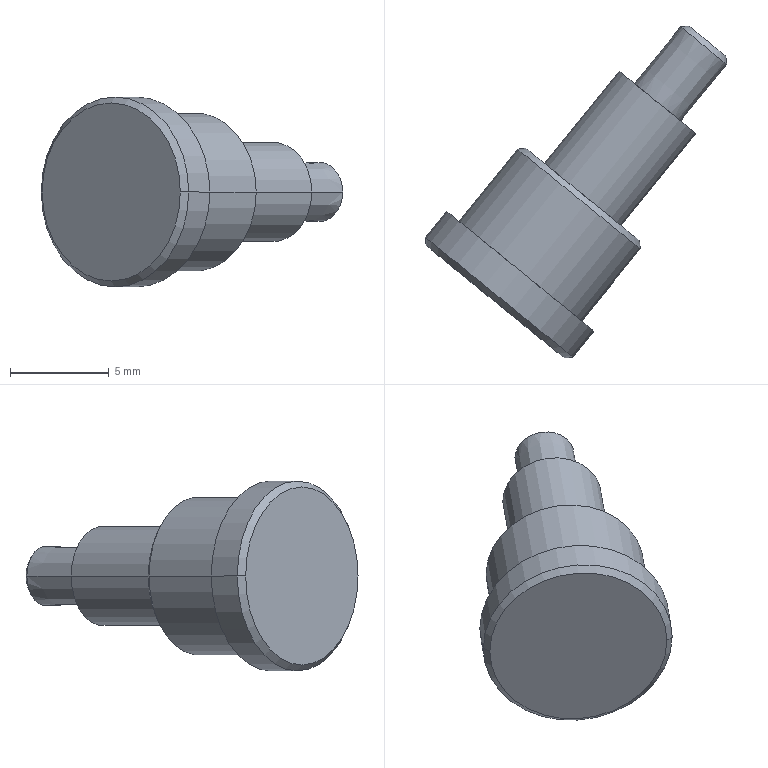Part | SolidWorks | features BaseBody 1 | 1 solid | 19 faces | box 15.235 x 16.785 x 9.6 mm | volume 539.336 mm3 | cone 8 | cylinder 6 | plane 5 | commonest cylinder face diameters 5 x2 8 x2 9.6 x2
STEP:
#1=CARTESIAN_POINT('',(528.138,-164.807,289.195));
#2=VERTEX_POINT('',#1);
#3=CARTESIAN_POINT('',(521.155,-159.129,289.195));
#4=VERTEX_POINT('',#3);
#5=CARTESIAN_POINT('',(524.647,-161.968,289.195));
#6=DIRECTION('',(-0.6309,-0.7758,0.000000012));
#7=DIRECTION('',(-0.7758,0.6309,0.));
#8=AXIS2_PLACEMENT_3D('',#5,#6,#7);
#9=CIRCLE('',#8,4.5);
#10=EDGE_CURVE('',#2,#4,#9,.T.);
#11=ORIENTED_EDGE('',*,*,#10,.F.);
#12=CARTESIAN_POINT('',(528.56,-164.764,289.195));
#13=VERTEX_POINT('',#12);
#14=CARTESIAN_POINT('',(528.56,-164.764,289.195));
#15=DIRECTION('',(0.9947,0.1025,-0.000000009));
#16=VECTOR('',#15,1000.);
#17=LINE('',#14,#16);
#18=EDGE_CURVE('',#2,#13,#17,.T.);
#19=ORIENTED_EDGE('',*,*,#18,.T.);
#20=CARTESIAN_POINT('',(521.112,-158.707,289.195));
#21=VERTEX_POINT('',#20);
#22=CARTESIAN_POINT('',(524.836,-161.736,289.195));
#23=DIRECTION('',(-0.6309,-0.7758,0.000000012));
#24=DIRECTION('',(0.7758,-0.6309,-0.000000021));
#25=AXIS2_PLACEMENT_3D('',#22,#23,#24);
#26=CIRCLE('',#25,4.8);
#27=EDGE_CURVE('',#13,#21,#26,.T.);
#28=ORIENTED_EDGE('',*,*,#27,.T.);
#29=CARTESIAN_POINT('',(521.112,-158.707,289.195));
#30=DIRECTION('',(-0.1025,0.9947,-0.000000009));
#31=VECTOR('',#30,1000.);
#32=LINE('',#29,#31);
#33=EDGE_CURVE('',#4,#21,#32,.T.);
#34=ORIENTED_EDGE('',*,*,#33,.F.);
#35=EDGE_LOOP('',(#11,#19,#28,#34));
#36=FACE_OUTER_BOUND('',#35,.T.);
#37=CARTESIAN_POINT('',(524.836,-161.736,289.195));
#38=DIRECTION('',(0.6309,0.7758,-0.000000012));
#39=DIRECTION('',(-0.7758,0.6309,0.));
#40=AXIS2_PLACEMENT_3D('',#37,#38,#39);
#41=CONICAL_SURFACE('',#40,4.8,0.7854);
#42=ADVANCED_FACE('',(#36),#41,.T.);
#43=ORIENTED_EDGE('',*,*,#27,.F.);
#44=CARTESIAN_POINT('',(529.633,-163.445,289.195));
#45=VERTEX_POINT('',#44);
#46=CARTESIAN_POINT('',(529.002,-164.221,289.195));
#47=DIRECTION('',(0.6309,0.7758,-0.000000012));
#48=VECTOR('',#47,1000.);
#49=LINE('',#46,#48);
#50=EDGE_CURVE('',#13,#45,#49,.T.);
#51=ORIENTED_EDGE('',*,*,#50,.T.);
#52=CARTESIAN_POINT('',(522.184,-157.388,289.195));
#53=VERTEX_POINT('',#52);
#54=CARTESIAN_POINT('',(525.908,-160.417,289.195));
#55=DIRECTION('',(-0.6309,-0.7758,0.000000012));
#56=DIRECTION('',(-0.7758,0.6309,0.));
#57=AXIS2_PLACEMENT_3D('',#54,#55,#56);
#58=CIRCLE('',#57,4.8);
#59=EDGE_CURVE('',#45,#53,#58,.T.);
#60=ORIENTED_EDGE('',*,*,#59,.T.);
#61=CARTESIAN_POINT('',(521.554,-158.164,289.195));
#62=DIRECTION('',(0.6309,0.7758,-0.000000012));
#63=VECTOR('',#62,1000.);
#64=LINE('',#61,#63);
#65=EDGE_CURVE('',#21,#53,#64,.T.);
#66=ORIENTED_EDGE('',*,*,#65,.F.);
#67=EDGE_LOOP('',(#43,#51,#60,#66));
#68=FACE_OUTER_BOUND('',#67,.T.);
#69=CARTESIAN_POINT('',(525.278,-161.192,289.195));
#70=DIRECTION('',(0.6309,0.7758,-0.000000012));
#71=DIRECTION('',(-0.7758,0.6309,0.));
#72=AXIS2_PLACEMENT_3D('',#69,#70,#71);
#73=CYLINDRICAL_SURFACE('',#72,4.8);
#74=ADVANCED_FACE('',(#68),#73,.T.);
#75=CARTESIAN_POINT('',(529.012,-162.94,289.195));
#76=VERTEX_POINT('',#75);
#77=CARTESIAN_POINT('',(522.805,-157.893,289.195));
#78=VERTEX_POINT('',#77);
#79=CARTESIAN_POINT('',(525.908,-160.417,289.195));
#80=DIRECTION('',(-0.6309,-0.7758,0.000000012));
#81=DIRECTION('',(-0.7758,0.6309,0.));
#82=AXIS2_PLACEMENT_3D('',#79,#80,#81);
#83=CIRCLE('',#82,4.);
#84=EDGE_CURVE('',#76,#78,#83,.T.);
#85=ORIENTED_EDGE('',*,*,#84,.F.);
#86=CARTESIAN_POINT('',(531.977,-159.294,289.195));
#87=VERTEX_POINT('',#86);
#88=CARTESIAN_POINT('',(530.589,-161.001,289.195));
#89=DIRECTION('',(0.6309,0.7758,-0.000000012));
#90=VECTOR('',#89,1000.);
#91=LINE('',#88,#90);
#92=EDGE_CURVE('',#76,#87,#91,.T.);
#93=ORIENTED_EDGE('',*,*,#92,.T.);
#94=CARTESIAN_POINT('',(525.77,-154.246,289.195));
#95=VERTEX_POINT('',#94);
#96=CARTESIAN_POINT('',(528.874,-156.77,289.195));
#97=DIRECTION('',(-0.6309,-0.7758,0.000000012));
#98=DIRECTION('',(-0.7758,0.6309,0.));
#99=AXIS2_PLACEMENT_3D('',#96,#97,#98);
#100=CIRCLE('',#99,4.);
#101=EDGE_CURVE('',#87,#95,#100,.T.);
#102=ORIENTED_EDGE('',*,*,#101,.T.);
#103=CARTESIAN_POINT('',(524.382,-155.953,289.195));
#104=DIRECTION('',(0.6309,0.7758,-0.000000012));
#105=VECTOR('',#104,1000.);
#106=LINE('',#103,#105);
#107=EDGE_CURVE('',#78,#95,#106,.T.);
#108=ORIENTED_EDGE('',*,*,#107,.F.);
#109=EDGE_LOOP('',(#85,#93,#102,#108));
#110=FACE_OUTER_BOUND('',#109,.T.);
#111=CARTESIAN_POINT('',(527.486,-158.477,289.195));
#112=DIRECTION('',(0.6309,0.7758,-0.000000012));
#113=DIRECTION('',(-0.7758,0.6309,0.));
#114=AXIS2_PLACEMENT_3D('',#111,#112,#113);
#115=CYLINDRICAL_SURFACE('',#114,4.);
#116=ADVANCED_FACE('',(#110),#115,.T.);
#117=CARTESIAN_POINT('',(531.934,-158.872,289.195));
#118=VERTEX_POINT('',#117);
#119=CARTESIAN_POINT('',(526.193,-154.203,289.195));
#120=VERTEX_POINT('',#119);
#121=CARTESIAN_POINT('',(529.063,-156.537,289.195));
#122=DIRECTION('',(-0.6309,-0.7758,0.000000012));
#123=DIRECTION('',(0.7758,-0.6309,0.));
#124=AXIS2_PLACEMENT_3D('',#121,#122,#123);
#125=CIRCLE('',#124,3.7);
#126=EDGE_CURVE('',#118,#120,#125,.T.);
#127=ORIENTED_EDGE('',*,*,#126,.T.);
#128=CARTESIAN_POINT('',(525.77,-154.246,289.195));
#129=DIRECTION('',(-0.9947,-0.1025,0.000000009));
#130=VECTOR('',#129,1000.);
#131=LINE('',#128,#130);
#132=EDGE_CURVE('',#120,#95,#131,.T.);
#133=ORIENTED_EDGE('',*,*,#132,.T.);
#134=ORIENTED_EDGE('',*,*,#101,.F.);
#135=CARTESIAN_POINT('',(531.977,-159.294,289.195));
#136=DIRECTION('',(0.1025,-0.9947,0.000000009));
#137=VECTOR('',#136,1000.);
#138=LINE('',#135,#137);
#139=EDGE_CURVE('',#118,#87,#138,.T.);
#140=ORIENTED_EDGE('',*,*,#139,.F.);
#141=EDGE_LOOP('',(#127,#133,#134,#140));
#142=FACE_OUTER_BOUND('',#141,.T.);
#143=CARTESIAN_POINT('',(528.874,-156.77,289.195));
#144=DIRECTION('',(-0.6309,-0.7758,0.000000012));
#145=DIRECTION('',(0.7758,-0.6309,0.));
#146=AXIS2_PLACEMENT_3D('',#143,#144,#145);
#147=CONICAL_SURFACE('',#146,4.,0.7854);
#148=ADVANCED_FACE('',(#142),#147,.T.);
#149=CARTESIAN_POINT('',(531.003,-158.115,289.195));
#150=VERTEX_POINT('',#149);
#151=CARTESIAN_POINT('',(527.124,-154.96,289.195));
#152=VERTEX_POINT('',#151);
#153=CARTESIAN_POINT('',(529.063,-156.537,289.195));
#154=DIRECTION('',(-0.6309,-0.7758,0.000000012));
#155=DIRECTION('',(-0.7758,0.6309,0.));
#156=AXIS2_PLACEMENT_3D('',#153,#154,#155);
#157=CIRCLE('',#156,2.5);
#158=EDGE_CURVE('',#150,#152,#157,.T.);
#159=ORIENTED_EDGE('',*,*,#158,.F.);
#160=CARTESIAN_POINT('',(534.788,-153.46,289.195));
#161=VERTEX_POINT('',#160);
#162=CARTESIAN_POINT('',(532.896,-155.787,289.195));
#163=DIRECTION('',(0.6309,0.7758,-0.000000012));
#164=VECTOR('',#163,1000.);
#165=LINE('',#162,#164);
#166=EDGE_CURVE('',#150,#161,#165,.T.);
#167=ORIENTED_EDGE('',*,*,#166,.T.);
#168=CARTESIAN_POINT('',(530.909,-150.305,289.195));
#169=VERTEX_POINT('',#168);
#170=CARTESIAN_POINT('',(532.849,-151.882,289.195));
#171=DIRECTION('',(-0.6309,-0.7758,0.000000012));
#172=DIRECTION('',(-0.7758,0.6309,0.));
#173=AXIS2_PLACEMENT_3D('',#170,#171,#172);
#174=CIRCLE('',#173,2.5);
#175=EDGE_CURVE('',#161,#169,#174,.T.);
#176=ORIENTED_EDGE('',*,*,#175,.T.);
#177=CARTESIAN_POINT('',(529.016,-152.633,289.195));
#178=DIRECTION('',(0.6309,0.7758,-0.000000012));
#179=VECTOR('',#178,1000.);
#180=LINE('',#177,#179);
#181=EDGE_CURVE('',#152,#169,#180,.T.);
#182=ORIENTED_EDGE('',*,*,#181,.F.);
#183=EDGE_LOOP('',(#159,#167,#176,#182));
#184=FACE_OUTER_BOUND('',#183,.T.);
#185=CARTESIAN_POINT('',(530.956,-154.21,289.195));
#186=DIRECTION('',(0.6309,0.7758,-0.000000012));
#187=DIRECTION('',(-0.7758,0.6309,0.));
#188=AXIS2_PLACEMENT_3D('',#185,#186,#187);
#189=CYLINDRICAL_SURFACE('',#188,2.5);
#190=ADVANCED_FACE('',(#184),#189,.T.);
#191=CARTESIAN_POINT('',(536.346,-149.958,289.195));
#192=VERTEX_POINT('',#191);
#193=CARTESIAN_POINT('',(534.02,-148.066,289.195));
#194=VERTEX_POINT('',#193);
#195=CARTESIAN_POINT('',(535.183,-149.012,289.195));
#196=DIRECTION('',(-0.6309,-0.7758,0.000000012));
#197=DIRECTION('',(0.7758,-0.6309,-0.000000021));
#198=AXIS2_PLACEMENT_3D('',#195,#196,#197);
#199=CIRCLE('',#198,1.499);
#200=EDGE_CURVE('',#192,#194,#199,.T.);
#201=ORIENTED_EDGE('',*,*,#200,.T.);
#202=CARTESIAN_POINT('',(531.685,-150.936,289.195));
#203=VERTEX_POINT('',#202);
#204=CARTESIAN_POINT('',(531.685,-150.936,289.195));
#205=DIRECTION('',(-0.6311,-0.7757,0.000000012));
#206=VECTOR('',#205,1000.);
#207=LINE('',#204,#206);
#208=EDGE_CURVE('',#194,#203,#207,.T.);
#209=ORIENTED_EDGE('',*,*,#208,.T.);
#210=CARTESIAN_POINT('',(534.012,-152.829,289.195));
#211=VERTEX_POINT('',#210);
#212=CARTESIAN_POINT('',(532.849,-151.882,289.195));
#213=DIRECTION('',(-0.6309,-0.7758,0.000000012));
#214=DIRECTION('',(0.7758,-0.6309,0.));
#215=AXIS2_PLACEMENT_3D('',#212,#213,#214);
#216=CIRCLE('',#215,1.5);
#217=EDGE_CURVE('',#211,#203,#216,.T.);
#218=ORIENTED_EDGE('',*,*,#217,.F.);
#219=CARTESIAN_POINT('',(534.012,-152.829,289.195));
#220=DIRECTION('',(-0.6308,-0.7759,0.000000012));
#221=VECTOR('',#220,1000.);
#222=LINE('',#219,#221);
#223=EDGE_CURVE('',#192,#211,#222,.T.);
#224=ORIENTED_EDGE('',*,*,#223,.F.);
#225=EDGE_LOOP('',(#201,#209,#218,#224));
#226=FACE_OUTER_BOUND('',#225,.T.);
#227=CARTESIAN_POINT('',(532.849,-151.882,289.195));
#228=DIRECTION('',(-0.6309,-0.7758,0.000000012));
#229=DIRECTION('',(0.7758,-0.6309,0.));
#230=AXIS2_PLACEMENT_3D('',#227,#228,#229);
#231=CONICAL_SURFACE('',#230,1.5,0.0001745);
#232=ADVANCED_FACE('',(#226),#231,.T.);
#233=CARTESIAN_POINT('',(536.303,-149.536,289.195));
#234=VERTEX_POINT('',#233);
#235=CARTESIAN_POINT('',(534.442,-148.022,289.195));
#236=VERTEX_POINT('',#235);
#237=CARTESIAN_POINT('',(535.372,-148.779,289.195));
#238=DIRECTION('',(-0.6309,-0.7758,0.000000012));
#239=DIRECTION('',(0.7758,-0.6309,0.));
#240=AXIS2_PLACEMENT_3D('',#237,#238,#239);
#241=CIRCLE('',#240,1.199);
#242=EDGE_CURVE('',#234,#236,#241,.T.);
#243=ORIENTED_EDGE('',*,*,#242,.T.);
#244=CARTESIAN_POINT('',(534.02,-148.066,289.195));
#245=DIRECTION('',(-0.9947,-0.1024,0.000000009));
#246=VECTOR('',#245,1000.);
#247=LINE('',#244,#246);
#248=EDGE_CURVE('',#236,#194,#247,.T.);
#249=ORIENTED_EDGE('',*,*,#248,.T.);
#250=ORIENTED_EDGE('',*,*,#200,.F.);
#251=CARTESIAN_POINT('',(536.346,-149.958,289.195));
#252=DIRECTION('',(0.1026,-0.9947,0.000000009));
#253=VECTOR('',#252,1000.);
#254=LINE('',#251,#253);
#255=EDGE_CURVE('',#234,#192,#254,.T.);
#256=ORIENTED_EDGE('',*,*,#255,.F.);
#257=EDGE_LOOP('',(#243,#249,#250,#256));
#258=FACE_OUTER_BOUND('',#257,.T.);
#259=CARTESIAN_POINT('',(535.183,-149.012,289.195));
#260=DIRECTION('',(-0.6309,-0.7758,0.000000012));
#261=DIRECTION('',(0.7758,-0.6309,0.));
#262=AXIS2_PLACEMENT_3D('',#259,#260,#261);
#263=CONICAL_SURFACE('',#262,1.499,0.7855);
#264=ADVANCED_FACE('',(#258),#263,.T.);
#265=CARTESIAN_POINT('',(524.647,-161.968,289.195));
#266=DIRECTION('',(-0.6309,-0.7758,0.000000012));
#267=DIRECTION('',(-0.7758,0.6309,0.));
#268=AXIS2_PLACEMENT_3D('',#265,#266,#267);
#269=CIRCLE('',#268,4.5);
#270=EDGE_CURVE('',#4,#2,#269,.T.);
#271=ORIENTED_EDGE('',*,*,#270,.T.);
#272=ORIENTED_EDGE('',*,*,#10,.T.);
#273=EDGE_LOOP('',(#271,#272));
#274=FACE_OUTER_BOUND('',#273,.T.);
#275=CARTESIAN_POINT('',(526.509,-163.482,289.195));
#276=DIRECTION('',(-0.6309,-0.7758,0.000000012));
#277=DIRECTION('',(0.7758,-0.6309,0.));
#278=AXIS2_PLACEMENT_3D('',#275,#276,#277);
#279=PLANE('',#278);
#280=ADVANCED_FACE('',(#274),#279,.T.);
#281=ORIENTED_EDGE('',*,*,#18,.F.);
#282=ORIENTED_EDGE('',*,*,#270,.F.);
#283=ORIENTED_EDGE('',*,*,#33,.T.);
#284=CARTESIAN_POINT('',(524.836,-161.736,289.195));
#285=DIRECTION('',(-0.6309,-0.7758,0.000000012));
#286=DIRECTION('',(0.7758,-0.6309,-0.000000021));
#287=AXIS2_PLACEMENT_3D('',#284,#285,#286);
#288=CIRCLE('',#287,4.8);
#289=EDGE_CURVE('',#21,#13,#288,.T.);
#290=ORIENTED_EDGE('',*,*,#289,.T.);
#291=EDGE_LOOP('',(#281,#282,#283,#290));
#292=FACE_OUTER_BOUND('',#291,.T.);
#293=CARTESIAN_POINT('',(524.836,-161.736,289.195));
#294=DIRECTION('',(0.6309,0.7758,-0.000000012));
#295=DIRECTION('',(-0.7758,0.6309,0.));
#296=AXIS2_PLACEMENT_3D('',#293,#294,#295);
#297=CONICAL_SURFACE('',#296,4.8,0.7854);
#298=ADVANCED_FACE('',(#292),#297,.T.);
#299=ORIENTED_EDGE('',*,*,#50,.F.);
#300=ORIENTED_EDGE('',*,*,#289,.F.);
#301=ORIENTED_EDGE('',*,*,#65,.T.);
#302=CARTESIAN_POINT('',(525.908,-160.417,289.195));
#303=DIRECTION('',(-0.6309,-0.7758,0.000000012));
#304=DIRECTION('',(-0.7758,0.6309,0.));
#305=AXIS2_PLACEMENT_3D('',#302,#303,#304);
#306=CIRCLE('',#305,4.8);
#307=EDGE_CURVE('',#53,#45,#306,.T.);
#308=ORIENTED_EDGE('',*,*,#307,.T.);
#309=EDGE_LOOP('',(#299,#300,#301,#308));
#310=FACE_OUTER_BOUND('',#309,.T.);
#311=CARTESIAN_POINT('',(525.278,-161.192,289.195));
#312=DIRECTION('',(0.6309,0.7758,-0.000000012));
#313=DIRECTION('',(-0.7758,0.6309,0.));
#314=AXIS2_PLACEMENT_3D('',#311,#312,#313);
#315=CYLINDRICAL_SURFACE('',#314,4.8);
#316=ADVANCED_FACE('',(#310),#315,.T.);
#317=CARTESIAN_POINT('',(525.908,-160.417,289.195));
#318=DIRECTION('',(-0.6309,-0.7758,0.000000012));
#319=DIRECTION('',(-0.7758,0.6309,0.));
#320=AXIS2_PLACEMENT_3D('',#317,#318,#319);
#321=CIRCLE('',#320,4.);
#322=EDGE_CURVE('',#78,#76,#321,.T.);
#323=ORIENTED_EDGE('',*,*,#322,.T.);
#324=ORIENTED_EDGE('',*,*,#84,.T.);
#325=EDGE_LOOP('',(#323,#324));
#326=FACE_BOUND('',#325,.T.);
#327=ORIENTED_EDGE('',*,*,#307,.F.);
#328=ORIENTED_EDGE('',*,*,#59,.F.);
#329=EDGE_LOOP('',(#327,#328));
#330=FACE_OUTER_BOUND('',#329,.T.);
#331=CARTESIAN_POINT('',(529.322,-163.193,289.195));
#332=DIRECTION('',(0.6309,0.7758,-0.000000012));
#333=DIRECTION('',(-0.7758,0.6309,0.));
#334=AXIS2_PLACEMENT_3D('',#331,#332,#333);
#335=PLANE('',#334);
#336=ADVANCED_FACE('',(#326,#330),#335,.T.);
#337=ORIENTED_EDGE('',*,*,#92,.F.);
#338=ORIENTED_EDGE('',*,*,#322,.F.);
#339=ORIENTED_EDGE('',*,*,#107,.T.);
#340=CARTESIAN_POINT('',(528.874,-156.77,289.195));
#341=DIRECTION('',(-0.6309,-0.7758,0.000000012));
#342=DIRECTION('',(-0.7758,0.6309,0.));
#343=AXIS2_PLACEMENT_3D('',#340,#341,#342);
#344=CIRCLE('',#343,4.);
#345=EDGE_CURVE('',#95,#87,#344,.T.);
#346=ORIENTED_EDGE('',*,*,#345,.T.);
#347=EDGE_LOOP('',(#337,#338,#339,#346));
#348=FACE_OUTER_BOUND('',#347,.T.);
#349=CARTESIAN_POINT('',(527.486,-158.477,289.195));
#350=DIRECTION('',(0.6309,0.7758,-0.000000012));
#351=DIRECTION('',(-0.7758,0.6309,0.));
#352=AXIS2_PLACEMENT_3D('',#349,#350,#351);
#353=CYLINDRICAL_SURFACE('',#352,4.);
#354=ADVANCED_FACE('',(#348),#353,.T.);
#355=ORIENTED_EDGE('',*,*,#132,.F.);
#356=CARTESIAN_POINT('',(529.063,-156.537,289.195));
#357=DIRECTION('',(-0.6309,-0.7758,0.000000012));
#358=DIRECTION('',(0.7758,-0.6309,0.));
#359=AXIS2_PLACEMENT_3D('',#356,#357,#358);
#360=CIRCLE('',#359,3.7);
#361=EDGE_CURVE('',#120,#118,#360,.T.);
#362=ORIENTED_EDGE('',*,*,#361,.T.);
#363=ORIENTED_EDGE('',*,*,#139,.T.);
#364=ORIENTED_EDGE('',*,*,#345,.F.);
#365=EDGE_LOOP('',(#355,#362,#363,#364));
#366=FACE_OUTER_BOUND('',#365,.T.);
#367=CARTESIAN_POINT('',(528.874,-156.77,289.195));
#368=DIRECTION('',(-0.6309,-0.7758,0.000000012));
#369=DIRECTION('',(0.7758,-0.6309,0.));
#370=AXIS2_PLACEMENT_3D('',#367,#368,#369);
#371=CONICAL_SURFACE('',#370,4.,0.7854);
#372=ADVANCED_FACE('',(#366),#371,.T.);
#373=ORIENTED_EDGE('',*,*,#126,.F.);
#374=ORIENTED_EDGE('',*,*,#361,.F.);
#375=EDGE_LOOP('',(#373,#374));
#376=FACE_OUTER_BOUND('',#375,.T.);
#377=CARTESIAN_POINT('',(529.063,-156.537,289.195));
#378=DIRECTION('',(-0.6309,-0.7758,0.000000012));
#379=DIRECTION('',(-0.7758,0.6309,0.));
#380=AXIS2_PLACEMENT_3D('',#377,#378,#379);
#381=CIRCLE('',#380,2.5);
#382=EDGE_CURVE('',#152,#150,#381,.T.);
#383=ORIENTED_EDGE('',*,*,#382,.T.);
#384=ORIENTED_EDGE('',*,*,#158,.T.);
#385=EDGE_LOOP('',(#383,#384));
#386=FACE_BOUND('',#385,.T.);
#387=CARTESIAN_POINT('',(531.585,-158.588,289.195));
#388=DIRECTION('',(0.6309,0.7758,-0.000000012));
#389=DIRECTION('',(-0.7758,0.6309,0.));
#390=AXIS2_PLACEMENT_3D('',#387,#388,#389);
#391=PLANE('',#390);
#392=ADVANCED_FACE('',(#376,#386),#391,.T.);
#393=ORIENTED_EDGE('',*,*,#166,.F.);
#394=ORIENTED_EDGE('',*,*,#382,.F.);
#395=ORIENTED_EDGE('',*,*,#181,.T.);
#396=CARTESIAN_POINT('',(532.849,-151.882,289.195));
#397=DIRECTION('',(-0.6309,-0.7758,0.000000012));
#398=DIRECTION('',(-0.7758,0.6309,0.));
#399=AXIS2_PLACEMENT_3D('',#396,#397,#398);
#400=CIRCLE('',#399,2.5);
#401=EDGE_CURVE('',#169,#161,#400,.T.);
#402=ORIENTED_EDGE('',*,*,#401,.T.);
#403=EDGE_LOOP('',(#393,#394,#395,#402));
#404=FACE_OUTER_BOUND('',#403,.T.);
#405=CARTESIAN_POINT('',(530.956,-154.21,289.195));
#406=DIRECTION('',(0.6309,0.7758,-0.000000012));
#407=DIRECTION('',(-0.7758,0.6309,0.));
#408=AXIS2_PLACEMENT_3D('',#405,#406,#407);
#409=CYLINDRICAL_SURFACE('',#408,2.5);
#410=ADVANCED_FACE('',(#404),#409,.T.);
#411=ORIENTED_EDGE('',*,*,#401,.F.);
#412=ORIENTED_EDGE('',*,*,#175,.F.);
#413=EDGE_LOOP('',(#411,#412));
#414=FACE_OUTER_BOUND('',#413,.T.);
#415=ORIENTED_EDGE('',*,*,#217,.T.);
#416=CARTESIAN_POINT('',(532.849,-151.882,289.195));
#417=DIRECTION('',(-0.6309,-0.7758,0.000000012));
#418=DIRECTION('',(0.7758,-0.6309,0.));
#419=AXIS2_PLACEMENT_3D('',#416,#417,#418);
#420=CIRCLE('',#419,1.5);
#421=EDGE_CURVE('',#203,#211,#420,.T.);
#422=ORIENTED_EDGE('',*,*,#421,.T.);
#423=EDGE_LOOP('',(#415,#422));
#424=FACE_BOUND('',#423,.T.);
#425=CARTESIAN_POINT('',(533.819,-152.671,289.195));
#426=DIRECTION('',(0.6309,0.7758,-0.000000012));
#427=DIRECTION('',(-0.7758,0.6309,0.));
#428=AXIS2_PLACEMENT_3D('',#425,#426,#427);
#429=PLANE('',#428);
#430=ADVANCED_FACE('',(#414,#424),#429,.T.);
#431=ORIENTED_EDGE('',*,*,#208,.F.);
#432=CARTESIAN_POINT('',(535.183,-149.012,289.195));
#433=DIRECTION('',(-0.6309,-0.7758,0.000000012));
#434=DIRECTION('',(0.7758,-0.6309,-0.000000021));
#435=AXIS2_PLACEMENT_3D('',#432,#433,#434);
#436=CIRCLE('',#435,1.499);
#437=EDGE_CURVE('',#194,#192,#436,.T.);
#438=ORIENTED_EDGE('',*,*,#437,.T.);
#439=ORIENTED_EDGE('',*,*,#223,.T.);
#440=ORIENTED_EDGE('',*,*,#421,.F.);
#441=EDGE_LOOP('',(#431,#438,#439,#440));
#442=FACE_OUTER_BOUND('',#441,.T.);
#443=CARTESIAN_POINT('',(532.849,-151.882,289.195));
#444=DIRECTION('',(-0.6309,-0.7758,0.000000012));
#445=DIRECTION('',(0.7758,-0.6309,0.));
#446=AXIS2_PLACEMENT_3D('',#443,#444,#445);
#447=CONICAL_SURFACE('',#446,1.5,0.0001745);
#448=ADVANCED_FACE('',(#442),#447,.T.);
#449=ORIENTED_EDGE('',*,*,#248,.F.);
#450=CARTESIAN_POINT('',(535.372,-148.779,289.195));
#451=DIRECTION('',(-0.6309,-0.7758,0.000000012));
#452=DIRECTION('',(0.7758,-0.6309,0.));
#453=AXIS2_PLACEMENT_3D('',#450,#451,#452);
#454=CIRCLE('',#453,1.199);
#455=EDGE_CURVE('',#236,#234,#454,.T.);
#456=ORIENTED_EDGE('',*,*,#455,.T.);
#457=ORIENTED_EDGE('',*,*,#255,.T.);
#458=ORIENTED_EDGE('',*,*,#437,.F.);
#459=EDGE_LOOP('',(#449,#456,#457,#458));
#460=FACE_OUTER_BOUND('',#459,.T.);
#461=CARTESIAN_POINT('',(535.183,-149.012,289.195));
#462=DIRECTION('',(-0.6309,-0.7758,0.000000012));
#463=DIRECTION('',(0.7758,-0.6309,0.));
#464=AXIS2_PLACEMENT_3D('',#461,#462,#463);
#465=CONICAL_SURFACE('',#464,1.499,0.7855);
#466=ADVANCED_FACE('',(#460),#465,.T.);
#467=ORIENTED_EDGE('',*,*,#242,.F.);
#468=ORIENTED_EDGE('',*,*,#455,.F.);
#469=EDGE_LOOP('',(#467,#468));
#470=FACE_OUTER_BOUND('',#469,.T.);
#471=CARTESIAN_POINT('',(535.372,-148.779,289.195));
#472=DIRECTION('',(0.6309,0.7758,-0.000000012));
#473=DIRECTION('',(-0.7758,0.6309,0.));
#474=AXIS2_PLACEMENT_3D('',#471,#472,#473);
#475=PLANE('',#474);
#476=ADVANCED_FACE('',(#470),#475,.T.);
#477=CLOSED_SHELL('',(#42,#74,#116,#148,#190,#232,#264,#280,#298,#316,#336,#354,#372,#392,#410,#430,#448,#466,#476));
#478=MANIFOLD_SOLID_BREP('',#477);
#479=CARTESIAN_POINT('',(0.,0.,0.));
#480=DIRECTION('',(0.,0.,1.));
#481=DIRECTION('',(1.,0.,0.));
#482=AXIS2_PLACEMENT_3D('',#479,#480,#481);
#483=(LENGTH_UNIT()NAMED_UNIT(*)SI_UNIT(.MILLI.,.METRE.));
#484=UNCERTAINTY_MEASURE_WITH_UNIT(LENGTH_MEASURE(0.00001),#483,'','');
#485=(NAMED_UNIT(*)PLANE_ANGLE_UNIT()SI_UNIT($,.RADIAN.));
#486=(NAMED_UNIT(*)SI_UNIT($,.STERADIAN.)SOLID_ANGLE_UNIT());
#487=(GEOMETRIC_REPRESENTATION_CONTEXT(3)GLOBAL_UNCERTAINTY_ASSIGNED_CONTEXT((#484))GLOBAL_UNIT_ASSIGNED_CONTEXT((#483,#485,#486))REPRESENTATION_CONTEXT('',''));
#488=ADVANCED_BREP_SHAPE_REPRESENTATION('',(#478,#482),#487);